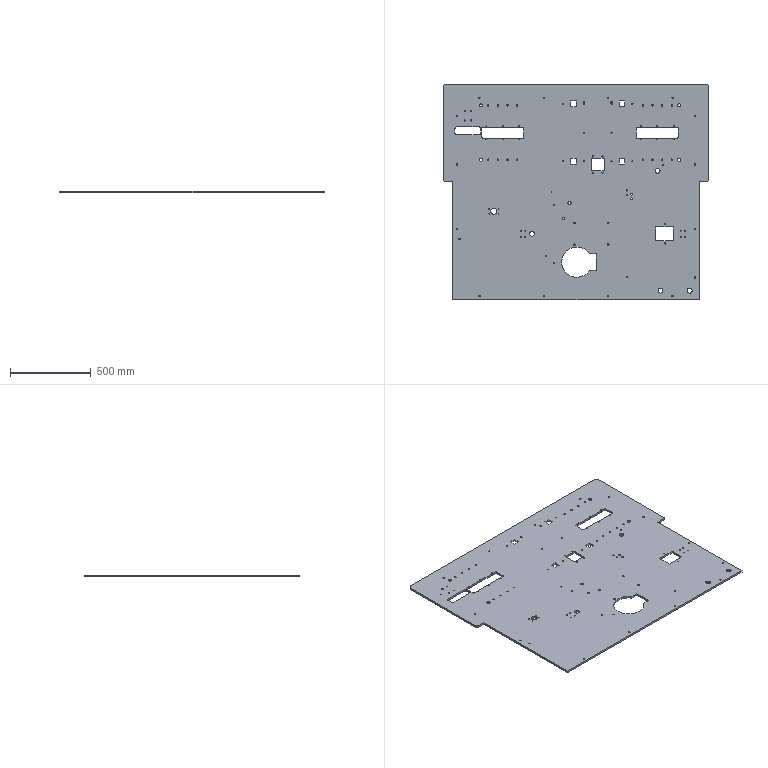Part | 1 solid | 272 faces | box 1650 x 1340 x 12 mm | volume 24180745 mm3 | cylinder 223 | plane 49 | commonest cylinder face diameters 6.8 x88 9 x62 20 x16 8.6 x12 3.3 x8 10 x8